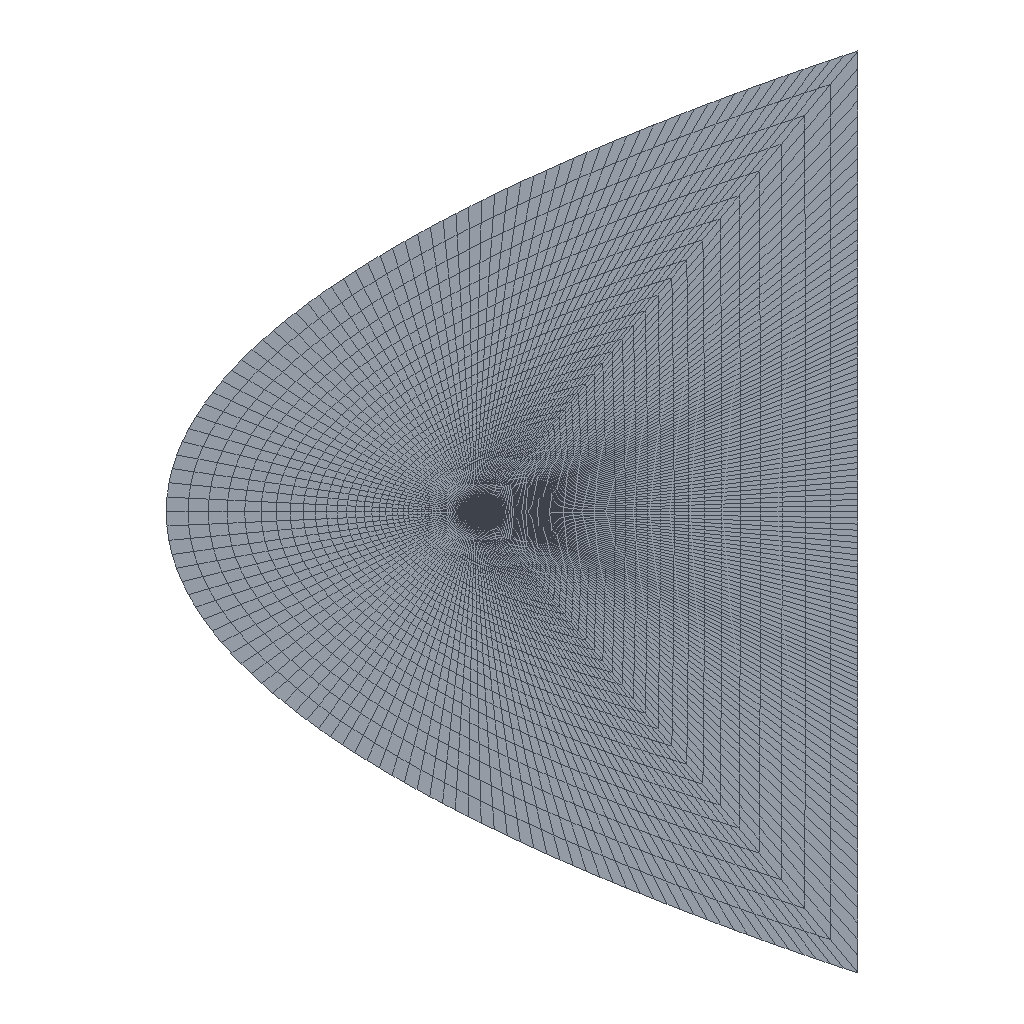Simulation study | ansys fluent
Set-up summary:
category,name,step,type,value,unit,region
solver,ansys_fluent,,Fluent 26.1.0
units,SI m-kg-s (Fluent internal),,stated,boundary values in the units shown in brackets; results in listed units
analysis,deck-1.cas,,cfd steady,"dimension=2D; solver=2d, dp, pbns, S-A (2d, double precision, pressure-based, Spalart-Allmaras); source_case=2.cas"
model,Space,deck-1.cas,,2D
model,Time,deck-1.cas,,Steady
model,Viscous,deck-1.cas,,Spalart-Allmaras turbulence model
model,Production Option,deck-1.cas,,Vorticity
model,Heat Transfer,deck-1.cas,,Enabled
model,Multiphase,deck-1.cas,,Disabled
analysis,deck-2.cas,,cfd steady,"dimension=2D; solver=2d, dp, pbns, S-A (2d, double precision, pressure-based, Spalart-Allmaras); source_case=.cas.h5"
model,Space,deck-2.cas,,2D
model,Time,deck-2.cas,,Steady
model,Viscous,deck-2.cas,,Spalart-Allmaras turbulence model
model,Production Option,deck-2.cas,,Vorticity
model,Heat Transfer,deck-2.cas,,Enabled
model,Multiphase,deck-2.cas,,Disabled
mesh,deck-1.cas,,nodes,37030
mesh,deck-1.cas,,elements,36800
mesh,deck-1.cas,,faces,73830
mesh,deck-1.cas,,note,elements = cells; counts from the case file zone headers
mesh,deck-2.cas,,nodes,37030
mesh,deck-2.cas,,elements,36800
mesh,deck-2.cas,,faces,73830
mesh,deck-2.cas,,note,elements = cells; counts from the case file zone headers
cell_zone,fluid,deck-1.cas,fluid,material=air,,zone 2
cell_zone,fluid,deck-2.cas,fluid,material=air,,zone 2
material,air (fluid),,Density,ideal-gas: #f,kg/m^3
material,air (fluid),,Cp (Specific Heat),1006.43,J/(kg K)
material,air (fluid),,Thermal Conductivity,0.0242,W/(m K)
material,air (fluid),,Viscosity,sutherland: (1.716e-05 273.11 110.56 ),kg/(m s)
material,air (fluid),,Molecular Weight,28.966,kg/kmol
material,aluminum (solid),,Density,2719,kg/m^3
material,aluminum (solid),,Cp (Specific Heat),871,J/(kg K)
material,aluminum (solid),,Thermal Conductivity,202.4,W/(m K)
bc,farfield,deck-1.cas,pressure-far-field,Mach Number=0.8; X-Component of Flow Direction=0.9976; Y-Component of Flow Direction=0.06976,,zone 3
bc,airfoil_upper,deck-1.cas,wall,Material Name=aluminum; Thermal BC Type=Heat Flux; Wall Motion=Stationary Wall; Shear Boundary Condition=No Slip; Wall Surface Roughness=Standard,,zone 4
bc,airfoil_lower,deck-1.cas,wall,Material Name=aluminum; Thermal BC Type=Heat Flux; Wall Motion=Stationary Wall; Shear Boundary Condition=No Slip; Wall Surface Roughness=Standard,,zone 5
bc,farfield,deck-2.cas,pressure-far-field,Mach Number=0.8; X-Component of Flow Direction=0.9976; Y-Component of Flow Direction=0.06976,,zone 3
bc,airfoil_upper,deck-2.cas,wall,Material Name=aluminum; Thermal BC Type=Heat Flux; Wall Motion=Stationary Wall; Shear Boundary Condition=No Slip; Wall Surface Roughness=Standard,,zone 4
bc,airfoil_lower,deck-2.cas,wall,Material Name=aluminum; Thermal BC Type=Heat Flux; Wall Motion=Stationary Wall; Shear Boundary Condition=No Slip; Wall Surface Roughness=Standard,,zone 5
Results summary:
result,mass flow rate airfoil_lower,deck-1.cas,,-0,kg/s
result,mass flow rate airfoil_upper,deck-1.cas,,-0,kg/s
result,mass flow rate farfield,deck-1.cas,,0.004041,kg/s
result,mass flow rate Net,deck-1.cas,,0.004041,kg/s
result,heat transfer rate airfoil_lower,deck-1.cas,,-0,W
result,heat transfer rate airfoil_upper,deck-1.cas,,-0,W
result,heat transfer rate farfield,deck-1.cas,,-1439.11,W
result,heat transfer rate Net,deck-1.cas,,-1439.11,W
result,wall force total airfoil_lower,deck-1.cas,,"(1676.75, -9990.15, 0)",N
result,wall force pressure airfoil_lower,deck-1.cas,,"(1538.83, -9989.06, 0)",N
result,wall force viscous airfoil_lower,deck-1.cas,,"(137.925, -1.085, 0)",N
result,wall force total airfoil_upper,deck-1.cas,,"(-350.196, 27181.4, 0)",N
result,wall force pressure airfoil_upper,deck-1.cas,,"(-425.084, 27167.6, 0)",N
result,wall force viscous airfoil_upper,deck-1.cas,,"(74.888, 13.81, 0)",N
result,wall force total Net,deck-1.cas,,"(1326.56, 17191.3, 0)",N
result,wall force pressure Net,deck-1.cas,,"(1113.75, 17178.6, 0)",N
result,wall force viscous Net,deck-1.cas,,"(212.813, 12.725, 0)",N
result,mass flow rate airfoil_lower,deck-2.cas,,-0,kg/s
result,mass flow rate airfoil_upper,deck-2.cas,,-0,kg/s
result,mass flow rate farfield,deck-2.cas,,0.004041,kg/s
result,mass flow rate Net,deck-2.cas,,0.004041,kg/s
result,heat transfer rate airfoil_lower,deck-2.cas,,-0,W
result,heat transfer rate airfoil_upper,deck-2.cas,,-0,W
result,heat transfer rate farfield,deck-2.cas,,-1439.11,W
result,heat transfer rate Net,deck-2.cas,,-1439.11,W
result,wall force total airfoil_lower,deck-2.cas,,"(1676.75, -9990.15, 0)",N
result,wall force pressure airfoil_lower,deck-2.cas,,"(1538.83, -9989.06, 0)",N
result,wall force viscous airfoil_lower,deck-2.cas,,"(137.925, -1.085, 0)",N
result,wall force total airfoil_upper,deck-2.cas,,"(-350.196, 27181.4, 0)",N
result,wall force pressure airfoil_upper,deck-2.cas,,"(-425.084, 27167.6, 0)",N
result,wall force viscous airfoil_upper,deck-2.cas,,"(74.888, 13.81, 0)",N
result,wall force total Net,deck-2.cas,,"(1326.56, 17191.3, 0)",N
result,wall force pressure Net,deck-2.cas,,"(1113.75, 17178.6, 0)",N
result,wall force viscous Net,deck-2.cas,,"(212.813, 12.725, 0)",N